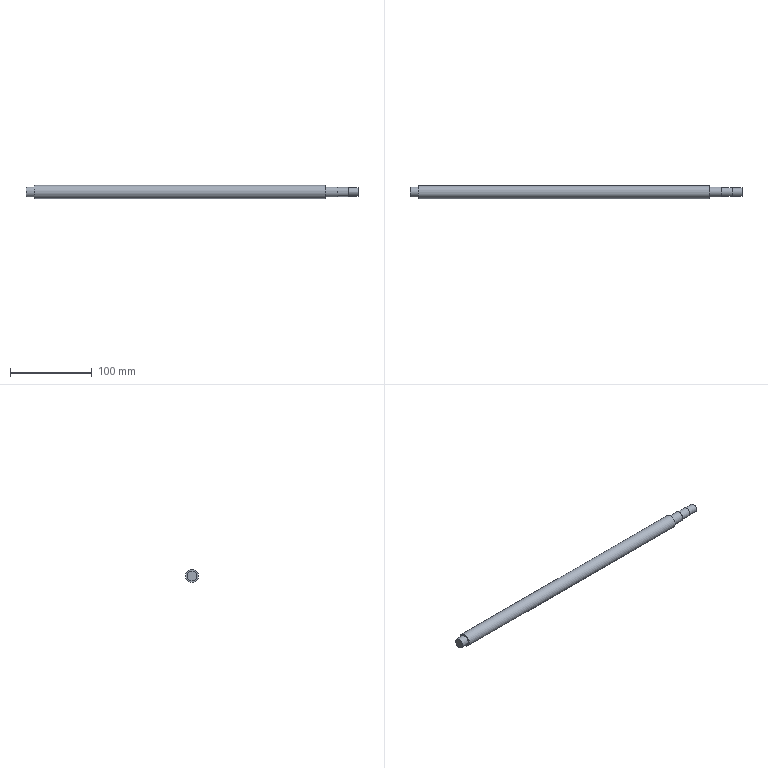Part | NX | 1 solid | 11 faces | box 405 x 16 x 16 mm | volume 76382 mm3 | plane 6 | cylinder 5 | commonest cylinder face diameters 12 x2 10 x1 11 x1 16 x1
STEP:
#1=CARTESIAN_POINT('',(-10.,0.,-6.));
#2=VERTEX_POINT('',#1);
#3=CARTESIAN_POINT('',(-10.,0.,0.));
#4=DIRECTION('',(1.,0.,0.));
#5=DIRECTION('',(0.,0.,-1.));
#6=AXIS2_PLACEMENT_3D('',#3,#4,#5);
#7=CIRCLE('',#6,6.);
#8=EDGE_CURVE('',#2,#2,#7,.T.);
#9=ORIENTED_EDGE('',*,*,#8,.F.);
#10=EDGE_LOOP('',(#9));
#11=FACE_OUTER_BOUND('',#10,.T.);
#12=CARTESIAN_POINT('',(-10.,0.,6.));
#13=DIRECTION('',(-1.,0.,0.));
#14=DIRECTION('',(0.,0.,-1.));
#15=AXIS2_PLACEMENT_3D('',#12,#13,#14);
#16=PLANE('',#15);
#17=ADVANCED_FACE('',(#11),#16,.T.);
#18=CARTESIAN_POINT('',(395.,0.,-5.));
#19=VERTEX_POINT('',#18);
#20=CARTESIAN_POINT('',(395.,0.,0.));
#21=DIRECTION('',(1.,0.,0.));
#22=DIRECTION('',(0.,0.,-1.));
#23=AXIS2_PLACEMENT_3D('',#20,#21,#22);
#24=CIRCLE('',#23,5.);
#25=EDGE_CURVE('',#19,#19,#24,.T.);
#26=ORIENTED_EDGE('',*,*,#25,.T.);
#27=EDGE_LOOP('',(#26));
#28=FACE_OUTER_BOUND('',#27,.T.);
#29=CARTESIAN_POINT('',(395.,0.,0.));
#30=DIRECTION('',(1.,0.,0.));
#31=DIRECTION('',(0.,0.,1.));
#32=AXIS2_PLACEMENT_3D('',#29,#30,#31);
#33=PLANE('',#32);
#34=ADVANCED_FACE('',(#28),#33,.T.);
#35=CARTESIAN_POINT('',(383.,0.,-5.));
#36=VERTEX_POINT('',#35);
#37=CARTESIAN_POINT('',(383.,0.,0.));
#38=DIRECTION('',(1.,0.,0.));
#39=DIRECTION('',(0.,0.,-1.));
#40=AXIS2_PLACEMENT_3D('',#37,#38,#39);
#41=CIRCLE('',#40,5.);
#42=EDGE_CURVE('',#36,#36,#41,.T.);
#43=ORIENTED_EDGE('',*,*,#42,.T.);
#44=EDGE_LOOP('',(#43));
#45=FACE_BOUND('',#44,.T.);
#46=ORIENTED_EDGE('',*,*,#25,.F.);
#47=EDGE_LOOP('',(#46));
#48=FACE_BOUND('',#47,.T.);
#49=CARTESIAN_POINT('',(-10.,0.,0.));
#50=DIRECTION('',(1.,0.,0.));
#51=DIRECTION('',(0.,0.,1.));
#52=AXIS2_PLACEMENT_3D('',#49,#50,#51);
#53=CYLINDRICAL_SURFACE('',#52,5.);
#54=ADVANCED_FACE('',(#45,#48),#53,.T.);
#55=CARTESIAN_POINT('',(383.,0.,-5.5));
#56=VERTEX_POINT('',#55);
#57=CARTESIAN_POINT('',(383.,0.,0.));
#58=DIRECTION('',(1.,0.,0.));
#59=DIRECTION('',(0.,0.,-1.));
#60=AXIS2_PLACEMENT_3D('',#57,#58,#59);
#61=CIRCLE('',#60,5.5);
#62=EDGE_CURVE('',#56,#56,#61,.T.);
#63=ORIENTED_EDGE('',*,*,#62,.T.);
#64=EDGE_LOOP('',(#63));
#65=FACE_BOUND('',#64,.T.);
#66=ORIENTED_EDGE('',*,*,#42,.F.);
#67=EDGE_LOOP('',(#66));
#68=FACE_BOUND('',#67,.T.);
#69=CARTESIAN_POINT('',(383.,0.,5.));
#70=DIRECTION('',(1.,0.,0.));
#71=DIRECTION('',(0.,0.,1.));
#72=AXIS2_PLACEMENT_3D('',#69,#70,#71);
#73=PLANE('',#72);
#74=ADVANCED_FACE('',(#65,#68),#73,.T.);
#75=CARTESIAN_POINT('',(370.,0.,-5.5));
#76=VERTEX_POINT('',#75);
#77=CARTESIAN_POINT('',(370.,0.,0.));
#78=DIRECTION('',(1.,0.,0.));
#79=DIRECTION('',(0.,0.,-1.));
#80=AXIS2_PLACEMENT_3D('',#77,#78,#79);
#81=CIRCLE('',#80,5.5);
#82=EDGE_CURVE('',#76,#76,#81,.T.);
#83=ORIENTED_EDGE('',*,*,#82,.T.);
#84=EDGE_LOOP('',(#83));
#85=FACE_BOUND('',#84,.T.);
#86=ORIENTED_EDGE('',*,*,#62,.F.);
#87=EDGE_LOOP('',(#86));
#88=FACE_BOUND('',#87,.T.);
#89=CARTESIAN_POINT('',(-10.,0.,0.));
#90=DIRECTION('',(1.,0.,0.));
#91=DIRECTION('',(0.,0.,1.));
#92=AXIS2_PLACEMENT_3D('',#89,#90,#91);
#93=CYLINDRICAL_SURFACE('',#92,5.5);
#94=ADVANCED_FACE('',(#85,#88),#93,.T.);
#95=CARTESIAN_POINT('',(370.,0.,-6.));
#96=VERTEX_POINT('',#95);
#97=CARTESIAN_POINT('',(370.,0.,0.));
#98=DIRECTION('',(1.,0.,0.));
#99=DIRECTION('',(0.,0.,-1.));
#100=AXIS2_PLACEMENT_3D('',#97,#98,#99);
#101=CIRCLE('',#100,6.);
#102=EDGE_CURVE('',#96,#96,#101,.T.);
#103=ORIENTED_EDGE('',*,*,#102,.T.);
#104=EDGE_LOOP('',(#103));
#105=FACE_BOUND('',#104,.T.);
#106=ORIENTED_EDGE('',*,*,#82,.F.);
#107=EDGE_LOOP('',(#106));
#108=FACE_BOUND('',#107,.T.);
#109=CARTESIAN_POINT('',(370.,0.,5.5));
#110=DIRECTION('',(1.,0.,0.));
#111=DIRECTION('',(0.,0.,1.));
#112=AXIS2_PLACEMENT_3D('',#109,#110,#111);
#113=PLANE('',#112);
#114=ADVANCED_FACE('',(#105,#108),#113,.T.);
#115=CARTESIAN_POINT('',(355.,0.,-6.));
#116=VERTEX_POINT('',#115);
#117=CARTESIAN_POINT('',(355.,0.,0.));
#118=DIRECTION('',(1.,0.,0.));
#119=DIRECTION('',(0.,0.,-1.));
#120=AXIS2_PLACEMENT_3D('',#117,#118,#119);
#121=CIRCLE('',#120,6.);
#122=EDGE_CURVE('',#116,#116,#121,.T.);
#123=ORIENTED_EDGE('',*,*,#122,.T.);
#124=EDGE_LOOP('',(#123));
#125=FACE_BOUND('',#124,.T.);
#126=ORIENTED_EDGE('',*,*,#102,.F.);
#127=EDGE_LOOP('',(#126));
#128=FACE_BOUND('',#127,.T.);
#129=CARTESIAN_POINT('',(-10.,0.,0.));
#130=DIRECTION('',(1.,0.,0.));
#131=DIRECTION('',(0.,0.,1.));
#132=AXIS2_PLACEMENT_3D('',#129,#130,#131);
#133=CYLINDRICAL_SURFACE('',#132,6.);
#134=ADVANCED_FACE('',(#125,#128),#133,.T.);
#135=CARTESIAN_POINT('',(355.,0.,-8.));
#136=VERTEX_POINT('',#135);
#137=CARTESIAN_POINT('',(355.,0.,0.));
#138=DIRECTION('',(1.,0.,0.));
#139=DIRECTION('',(0.,0.,-1.));
#140=AXIS2_PLACEMENT_3D('',#137,#138,#139);
#141=CIRCLE('',#140,8.);
#142=EDGE_CURVE('',#136,#136,#141,.T.);
#143=ORIENTED_EDGE('',*,*,#142,.T.);
#144=EDGE_LOOP('',(#143));
#145=FACE_BOUND('',#144,.T.);
#146=ORIENTED_EDGE('',*,*,#122,.F.);
#147=EDGE_LOOP('',(#146));
#148=FACE_BOUND('',#147,.T.);
#149=CARTESIAN_POINT('',(355.,0.,6.));
#150=DIRECTION('',(1.,0.,0.));
#151=DIRECTION('',(0.,0.,1.));
#152=AXIS2_PLACEMENT_3D('',#149,#150,#151);
#153=PLANE('',#152);
#154=ADVANCED_FACE('',(#145,#148),#153,.T.);
#155=CARTESIAN_POINT('',(0.,0.,-8.));
#156=VERTEX_POINT('',#155);
#157=CARTESIAN_POINT('',(0.,0.,0.));
#158=DIRECTION('',(1.,0.,0.));
#159=DIRECTION('',(0.,0.,-1.));
#160=AXIS2_PLACEMENT_3D('',#157,#158,#159);
#161=CIRCLE('',#160,8.);
#162=EDGE_CURVE('',#156,#156,#161,.T.);
#163=ORIENTED_EDGE('',*,*,#162,.T.);
#164=EDGE_LOOP('',(#163));
#165=FACE_BOUND('',#164,.T.);
#166=ORIENTED_EDGE('',*,*,#142,.F.);
#167=EDGE_LOOP('',(#166));
#168=FACE_BOUND('',#167,.T.);
#169=CARTESIAN_POINT('',(-10.,0.,0.));
#170=DIRECTION('',(1.,0.,0.));
#171=DIRECTION('',(0.,0.,1.));
#172=AXIS2_PLACEMENT_3D('',#169,#170,#171);
#173=CYLINDRICAL_SURFACE('',#172,8.);
#174=ADVANCED_FACE('',(#165,#168),#173,.T.);
#175=CARTESIAN_POINT('',(0.,0.,-6.));
#176=VERTEX_POINT('',#175);
#177=CARTESIAN_POINT('',(0.,0.,0.));
#178=DIRECTION('',(1.,0.,0.));
#179=DIRECTION('',(0.,0.,-1.));
#180=AXIS2_PLACEMENT_3D('',#177,#178,#179);
#181=CIRCLE('',#180,6.);
#182=EDGE_CURVE('',#176,#176,#181,.T.);
#183=ORIENTED_EDGE('',*,*,#182,.T.);
#184=EDGE_LOOP('',(#183));
#185=FACE_BOUND('',#184,.T.);
#186=ORIENTED_EDGE('',*,*,#162,.F.);
#187=EDGE_LOOP('',(#186));
#188=FACE_BOUND('',#187,.T.);
#189=CARTESIAN_POINT('',(0.,0.,8.));
#190=DIRECTION('',(-1.,0.,0.));
#191=DIRECTION('',(0.,0.,-1.));
#192=AXIS2_PLACEMENT_3D('',#189,#190,#191);
#193=PLANE('',#192);
#194=ADVANCED_FACE('',(#185,#188),#193,.T.);
#195=ORIENTED_EDGE('',*,*,#8,.T.);
#196=EDGE_LOOP('',(#195));
#197=FACE_BOUND('',#196,.T.);
#198=ORIENTED_EDGE('',*,*,#182,.F.);
#199=EDGE_LOOP('',(#198));
#200=FACE_BOUND('',#199,.T.);
#201=CARTESIAN_POINT('',(-10.,0.,0.));
#202=DIRECTION('',(1.,0.,0.));
#203=DIRECTION('',(0.,0.,1.));
#204=AXIS2_PLACEMENT_3D('',#201,#202,#203);
#205=CYLINDRICAL_SURFACE('',#204,6.);
#206=ADVANCED_FACE('',(#197,#200),#205,.T.);
#207=CLOSED_SHELL('',(#17,#34,#54,#74,#94,#114,#134,#154,#174,#194,#206));
#208=MANIFOLD_SOLID_BREP('',#207);
#209=(LENGTH_UNIT()NAMED_UNIT(*)SI_UNIT(.MILLI.,.METRE.));
#210=UNCERTAINTY_MEASURE_WITH_UNIT(LENGTH_MEASURE(0.00002),#209,'','');
#211=(NAMED_UNIT(*)PLANE_ANGLE_UNIT()SI_UNIT($,.RADIAN.));
#212=PLANE_ANGLE_MEASURE_WITH_UNIT(PLANE_ANGLE_MEASURE(0.01745),#211);
#213=DIMENSIONAL_EXPONENTS(0.,0.,0.,0.,0.,0.,0.);
#214=(CONVERSION_BASED_UNIT('DEGREE',#212)NAMED_UNIT(#213)PLANE_ANGLE_UNIT());
#215=(NAMED_UNIT(*)SI_UNIT($,.STERADIAN.)SOLID_ANGLE_UNIT());
#216=(GEOMETRIC_REPRESENTATION_CONTEXT(3)GLOBAL_UNCERTAINTY_ASSIGNED_CONTEXT((#210))GLOBAL_UNIT_ASSIGNED_CONTEXT((#209,#214,#215))REPRESENTATION_CONTEXT('',''));
#217=ADVANCED_BREP_SHAPE_REPRESENTATION('',(#208),#216);